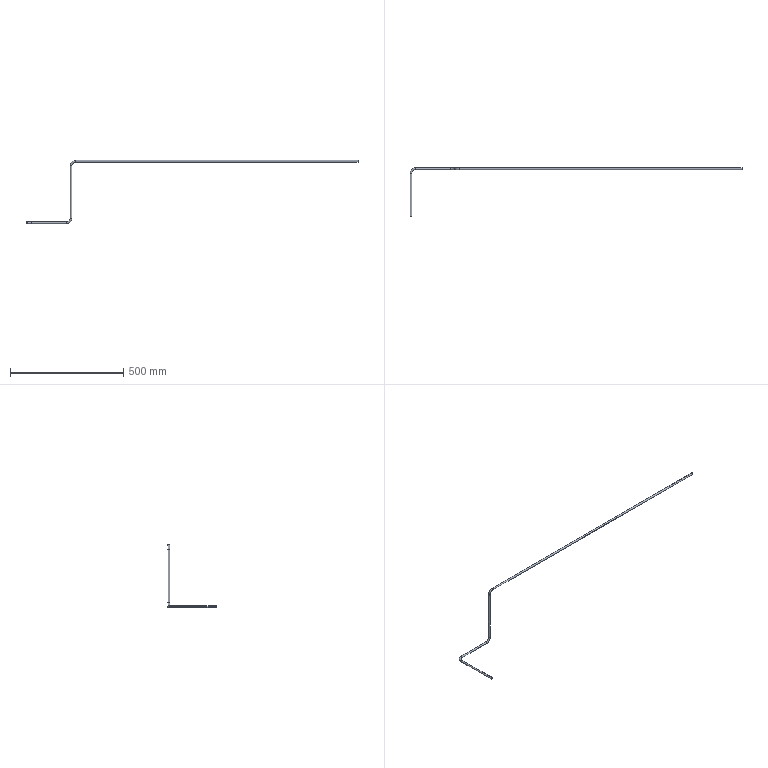Part | NX | features solid 2 | 1 solid | 16 faces | box 1467 x 214 x 279.213 mm | volume 82883 mm3 | cylinder 8 | torus 6 | plane 2 | commonest cylinder face diameters 3 x4 8 x4
STEP:
#1=CARTESIAN_POINT('',(-940.,-25.,-372.213));
#2=VERTEX_POINT('',#1);
#3=CARTESIAN_POINT('',(-940.,-25.,-376.213));
#4=DIRECTION('',(0.,-1.,0.));
#5=DIRECTION('',(0.,0.,1.));
#6=AXIS2_PLACEMENT_3D('',#3,#4,#5);
#7=CIRCLE('',#6,4.);
#8=EDGE_CURVE('',#2,#2,#7,.T.);
#9=ORIENTED_EDGE('',*,*,#8,.T.);
#10=EDGE_LOOP('',(#9));
#11=FACE_BOUND('',#10,.T.);
#12=CARTESIAN_POINT('',(-940.,-215.,-372.213));
#13=VERTEX_POINT('',#12);
#14=CARTESIAN_POINT('',(-940.,-215.,-376.213));
#15=DIRECTION('',(0.,-1.,0.));
#16=DIRECTION('',(0.,0.,1.));
#17=AXIS2_PLACEMENT_3D('',#14,#15,#16);
#18=CIRCLE('',#17,4.);
#19=EDGE_CURVE('',#13,#13,#18,.T.);
#20=ORIENTED_EDGE('',*,*,#19,.F.);
#21=EDGE_LOOP('',(#20));
#22=FACE_BOUND('',#21,.T.);
#23=CARTESIAN_POINT('',(-940.,-25.,-376.213));
#24=DIRECTION('',(0.,-1.,0.));
#25=DIRECTION('',(0.,0.,-1.));
#26=AXIS2_PLACEMENT_3D('',#23,#24,#25);
#27=CYLINDRICAL_SURFACE('',#26,4.);
#28=ADVANCED_FACE('',(#11,#22),#27,.T.);
#29=CARTESIAN_POINT('',(-940.,-25.,-374.713));
#30=VERTEX_POINT('',#29);
#31=CARTESIAN_POINT('',(-940.,-25.,-376.213));
#32=DIRECTION('',(0.,-1.,0.));
#33=DIRECTION('',(0.,0.,1.));
#34=AXIS2_PLACEMENT_3D('',#31,#32,#33);
#35=CIRCLE('',#34,1.5);
#36=EDGE_CURVE('',#30,#30,#35,.T.);
#37=ORIENTED_EDGE('',*,*,#36,.F.);
#38=EDGE_LOOP('',(#37));
#39=FACE_BOUND('',#38,.T.);
#40=CARTESIAN_POINT('',(-940.,-215.,-374.713));
#41=VERTEX_POINT('',#40);
#42=CARTESIAN_POINT('',(-940.,-215.,-376.213));
#43=DIRECTION('',(0.,-1.,0.));
#44=DIRECTION('',(0.,0.,1.));
#45=AXIS2_PLACEMENT_3D('',#42,#43,#44);
#46=CIRCLE('',#45,1.5);
#47=EDGE_CURVE('',#41,#41,#46,.T.);
#48=ORIENTED_EDGE('',*,*,#47,.T.);
#49=EDGE_LOOP('',(#48));
#50=FACE_BOUND('',#49,.T.);
#51=CARTESIAN_POINT('',(-940.,-25.,-376.213));
#52=DIRECTION('',(0.,-1.,0.));
#53=DIRECTION('',(0.,0.,-1.));
#54=AXIS2_PLACEMENT_3D('',#51,#52,#53);
#55=CYLINDRICAL_SURFACE('',#54,1.5);
#56=ADVANCED_FACE('',(#39,#50),#55,.F.);
#57=CARTESIAN_POINT('',(-920.,-5.,-372.213));
#58=VERTEX_POINT('',#57);
#59=CARTESIAN_POINT('',(-920.,-5.,-376.213));
#60=DIRECTION('',(-1.,0.,0.));
#61=DIRECTION('',(0.,0.,1.));
#62=AXIS2_PLACEMENT_3D('',#59,#60,#61);
#63=CIRCLE('',#62,4.);
#64=EDGE_CURVE('',#58,#58,#63,.T.);
#65=ORIENTED_EDGE('',*,*,#64,.T.);
#66=EDGE_LOOP('',(#65));
#67=FACE_BOUND('',#66,.T.);
#68=ORIENTED_EDGE('',*,*,#8,.F.);
#69=EDGE_LOOP('',(#68));
#70=FACE_BOUND('',#69,.T.);
#71=CARTESIAN_POINT('',(-920.,-25.,-376.213));
#72=DIRECTION('',(0.,0.,1.));
#73=DIRECTION('',(1.,0.,0.));
#74=AXIS2_PLACEMENT_3D('',#71,#72,#73);
#75=TOROIDAL_SURFACE('',#74,20.,4.);
#76=ADVANCED_FACE('',(#67,#70),#75,.T.);
#77=CARTESIAN_POINT('',(-920.,-5.,-374.713));
#78=VERTEX_POINT('',#77);
#79=CARTESIAN_POINT('',(-920.,-5.,-376.213));
#80=DIRECTION('',(-1.,0.,0.));
#81=DIRECTION('',(0.,0.,1.));
#82=AXIS2_PLACEMENT_3D('',#79,#80,#81);
#83=CIRCLE('',#82,1.5);
#84=EDGE_CURVE('',#78,#78,#83,.T.);
#85=ORIENTED_EDGE('',*,*,#84,.F.);
#86=EDGE_LOOP('',(#85));
#87=FACE_BOUND('',#86,.T.);
#88=ORIENTED_EDGE('',*,*,#36,.T.);
#89=EDGE_LOOP('',(#88));
#90=FACE_BOUND('',#89,.T.);
#91=CARTESIAN_POINT('',(-920.,-25.,-376.213));
#92=DIRECTION('',(0.,0.,1.));
#93=DIRECTION('',(1.,0.,0.));
#94=AXIS2_PLACEMENT_3D('',#91,#92,#93);
#95=TOROIDAL_SURFACE('',#94,20.,1.5);
#96=ADVANCED_FACE('',(#87,#90),#95,.F.);
#97=CARTESIAN_POINT('',(-765.,-5.,-372.213));
#98=VERTEX_POINT('',#97);
#99=CARTESIAN_POINT('',(-765.,-5.,-376.213));
#100=DIRECTION('',(-1.,0.,0.));
#101=DIRECTION('',(0.,0.,1.));
#102=AXIS2_PLACEMENT_3D('',#99,#100,#101);
#103=CIRCLE('',#102,4.);
#104=EDGE_CURVE('',#98,#98,#103,.T.);
#105=ORIENTED_EDGE('',*,*,#104,.T.);
#106=EDGE_LOOP('',(#105));
#107=FACE_BOUND('',#106,.T.);
#108=ORIENTED_EDGE('',*,*,#64,.F.);
#109=EDGE_LOOP('',(#108));
#110=FACE_BOUND('',#109,.T.);
#111=CARTESIAN_POINT('',(-765.,-5.,-376.213));
#112=DIRECTION('',(-1.,0.,0.));
#113=DIRECTION('',(0.,0.,1.));
#114=AXIS2_PLACEMENT_3D('',#111,#112,#113);
#115=CYLINDRICAL_SURFACE('',#114,4.);
#116=ADVANCED_FACE('',(#107,#110),#115,.T.);
#117=CARTESIAN_POINT('',(-765.,-5.,-374.713));
#118=VERTEX_POINT('',#117);
#119=CARTESIAN_POINT('',(-765.,-5.,-376.213));
#120=DIRECTION('',(-1.,0.,0.));
#121=DIRECTION('',(0.,0.,1.));
#122=AXIS2_PLACEMENT_3D('',#119,#120,#121);
#123=CIRCLE('',#122,1.5);
#124=EDGE_CURVE('',#118,#118,#123,.T.);
#125=ORIENTED_EDGE('',*,*,#124,.F.);
#126=EDGE_LOOP('',(#125));
#127=FACE_BOUND('',#126,.T.);
#128=ORIENTED_EDGE('',*,*,#84,.T.);
#129=EDGE_LOOP('',(#128));
#130=FACE_BOUND('',#129,.T.);
#131=CARTESIAN_POINT('',(-765.,-5.,-376.213));
#132=DIRECTION('',(-1.,0.,0.));
#133=DIRECTION('',(0.,0.,1.));
#134=AXIS2_PLACEMENT_3D('',#131,#132,#133);
#135=CYLINDRICAL_SURFACE('',#134,1.5);
#136=ADVANCED_FACE('',(#127,#130),#135,.F.);
#137=CARTESIAN_POINT('',(-749.,-5.,-356.213));
#138=VERTEX_POINT('',#137);
#139=CARTESIAN_POINT('',(-745.,-5.,-356.213));
#140=DIRECTION('',(0.,0.,-1.));
#141=DIRECTION('',(-1.,0.,0.));
#142=AXIS2_PLACEMENT_3D('',#139,#140,#141);
#143=CIRCLE('',#142,4.);
#144=EDGE_CURVE('',#138,#138,#143,.T.);
#145=ORIENTED_EDGE('',*,*,#144,.T.);
#146=EDGE_LOOP('',(#145));
#147=FACE_BOUND('',#146,.T.);
#148=ORIENTED_EDGE('',*,*,#104,.F.);
#149=EDGE_LOOP('',(#148));
#150=FACE_BOUND('',#149,.T.);
#151=CARTESIAN_POINT('',(-765.,-5.,-356.213));
#152=DIRECTION('',(0.,1.,0.));
#153=DIRECTION('',(0.,0.,1.));
#154=AXIS2_PLACEMENT_3D('',#151,#152,#153);
#155=TOROIDAL_SURFACE('',#154,20.,4.);
#156=ADVANCED_FACE('',(#147,#150),#155,.T.);
#157=CARTESIAN_POINT('',(-746.5,-5.,-356.213));
#158=VERTEX_POINT('',#157);
#159=CARTESIAN_POINT('',(-745.,-5.,-356.213));
#160=DIRECTION('',(0.,0.,-1.));
#161=DIRECTION('',(-1.,0.,0.));
#162=AXIS2_PLACEMENT_3D('',#159,#160,#161);
#163=CIRCLE('',#162,1.5);
#164=EDGE_CURVE('',#158,#158,#163,.T.);
#165=ORIENTED_EDGE('',*,*,#164,.F.);
#166=EDGE_LOOP('',(#165));
#167=FACE_BOUND('',#166,.T.);
#168=ORIENTED_EDGE('',*,*,#124,.T.);
#169=EDGE_LOOP('',(#168));
#170=FACE_BOUND('',#169,.T.);
#171=CARTESIAN_POINT('',(-765.,-5.,-356.213));
#172=DIRECTION('',(0.,1.,0.));
#173=DIRECTION('',(0.,0.,1.));
#174=AXIS2_PLACEMENT_3D('',#171,#172,#173);
#175=TOROIDAL_SURFACE('',#174,20.,1.5);
#176=ADVANCED_FACE('',(#167,#170),#175,.F.);
#177=CARTESIAN_POINT('',(-749.,-5.,-125.));
#178=VERTEX_POINT('',#177);
#179=CARTESIAN_POINT('',(-745.,-5.,-125.));
#180=DIRECTION('',(0.,0.,-1.));
#181=DIRECTION('',(-1.,0.,0.));
#182=AXIS2_PLACEMENT_3D('',#179,#180,#181);
#183=CIRCLE('',#182,4.);
#184=EDGE_CURVE('',#178,#178,#183,.T.);
#185=ORIENTED_EDGE('',*,*,#184,.T.);
#186=EDGE_LOOP('',(#185));
#187=FACE_BOUND('',#186,.T.);
#188=ORIENTED_EDGE('',*,*,#144,.F.);
#189=EDGE_LOOP('',(#188));
#190=FACE_BOUND('',#189,.T.);
#191=CARTESIAN_POINT('',(-745.,-5.,-125.));
#192=DIRECTION('',(0.,0.,-1.));
#193=DIRECTION('',(-1.,0.,0.));
#194=AXIS2_PLACEMENT_3D('',#191,#192,#193);
#195=CYLINDRICAL_SURFACE('',#194,4.);
#196=ADVANCED_FACE('',(#187,#190),#195,.T.);
#197=CARTESIAN_POINT('',(-746.5,-5.,-125.));
#198=VERTEX_POINT('',#197);
#199=CARTESIAN_POINT('',(-745.,-5.,-125.));
#200=DIRECTION('',(0.,0.,-1.));
#201=DIRECTION('',(-1.,0.,0.));
#202=AXIS2_PLACEMENT_3D('',#199,#200,#201);
#203=CIRCLE('',#202,1.5);
#204=EDGE_CURVE('',#198,#198,#203,.T.);
#205=ORIENTED_EDGE('',*,*,#204,.F.);
#206=EDGE_LOOP('',(#205));
#207=FACE_BOUND('',#206,.T.);
#208=ORIENTED_EDGE('',*,*,#164,.T.);
#209=EDGE_LOOP('',(#208));
#210=FACE_BOUND('',#209,.T.);
#211=CARTESIAN_POINT('',(-745.,-5.,-125.));
#212=DIRECTION('',(0.,0.,-1.));
#213=DIRECTION('',(-1.,0.,0.));
#214=AXIS2_PLACEMENT_3D('',#211,#212,#213);
#215=CYLINDRICAL_SURFACE('',#214,1.5);
#216=ADVANCED_FACE('',(#207,#210),#215,.F.);
#217=CARTESIAN_POINT('',(-725.,-5.,-101.));
#218=VERTEX_POINT('',#217);
#219=CARTESIAN_POINT('',(-725.,-5.,-105.));
#220=DIRECTION('',(-1.,0.,0.));
#221=DIRECTION('',(0.,0.,1.));
#222=AXIS2_PLACEMENT_3D('',#219,#220,#221);
#223=CIRCLE('',#222,4.);
#224=EDGE_CURVE('',#218,#218,#223,.T.);
#225=ORIENTED_EDGE('',*,*,#224,.T.);
#226=EDGE_LOOP('',(#225));
#227=FACE_BOUND('',#226,.T.);
#228=ORIENTED_EDGE('',*,*,#184,.F.);
#229=EDGE_LOOP('',(#228));
#230=FACE_BOUND('',#229,.T.);
#231=CARTESIAN_POINT('',(-725.,-5.,-125.));
#232=DIRECTION('',(0.,-1.,0.));
#233=DIRECTION('',(0.,0.,-1.));
#234=AXIS2_PLACEMENT_3D('',#231,#232,#233);
#235=TOROIDAL_SURFACE('',#234,20.,4.);
#236=ADVANCED_FACE('',(#227,#230),#235,.T.);
#237=CARTESIAN_POINT('',(-725.,-5.,-103.5));
#238=VERTEX_POINT('',#237);
#239=CARTESIAN_POINT('',(-725.,-5.,-105.));
#240=DIRECTION('',(-1.,0.,0.));
#241=DIRECTION('',(0.,0.,1.));
#242=AXIS2_PLACEMENT_3D('',#239,#240,#241);
#243=CIRCLE('',#242,1.5);
#244=EDGE_CURVE('',#238,#238,#243,.T.);
#245=ORIENTED_EDGE('',*,*,#244,.F.);
#246=EDGE_LOOP('',(#245));
#247=FACE_BOUND('',#246,.T.);
#248=ORIENTED_EDGE('',*,*,#204,.T.);
#249=EDGE_LOOP('',(#248));
#250=FACE_BOUND('',#249,.T.);
#251=CARTESIAN_POINT('',(-725.,-5.,-125.));
#252=DIRECTION('',(0.,-1.,0.));
#253=DIRECTION('',(0.,0.,-1.));
#254=AXIS2_PLACEMENT_3D('',#251,#252,#253);
#255=TOROIDAL_SURFACE('',#254,20.,1.5);
#256=ADVANCED_FACE('',(#247,#250),#255,.F.);
#257=ORIENTED_EDGE('',*,*,#244,.T.);
#258=EDGE_LOOP('',(#257));
#259=FACE_BOUND('',#258,.T.);
#260=CARTESIAN_POINT('',(523.271,-5.,-103.5));
#261=VERTEX_POINT('',#260);
#262=CARTESIAN_POINT('',(523.271,-5.,-105.));
#263=DIRECTION('',(-1.,0.,0.));
#264=DIRECTION('',(0.,0.,1.));
#265=AXIS2_PLACEMENT_3D('',#262,#263,#264);
#266=CIRCLE('',#265,1.5);
#267=EDGE_CURVE('',#261,#261,#266,.T.);
#268=ORIENTED_EDGE('',*,*,#267,.F.);
#269=EDGE_LOOP('',(#268));
#270=FACE_BOUND('',#269,.T.);
#271=CARTESIAN_POINT('',(-725.,-5.,-105.));
#272=DIRECTION('',(1.,0.,0.));
#273=DIRECTION('',(0.,0.,-1.));
#274=AXIS2_PLACEMENT_3D('',#271,#272,#273);
#275=CYLINDRICAL_SURFACE('',#274,1.5);
#276=ADVANCED_FACE('',(#259,#270),#275,.F.);
#277=ORIENTED_EDGE('',*,*,#224,.F.);
#278=EDGE_LOOP('',(#277));
#279=FACE_BOUND('',#278,.T.);
#280=CARTESIAN_POINT('',(523.271,-5.,-101.));
#281=VERTEX_POINT('',#280);
#282=CARTESIAN_POINT('',(523.271,-5.,-105.));
#283=DIRECTION('',(-1.,0.,0.));
#284=DIRECTION('',(0.,0.,1.));
#285=AXIS2_PLACEMENT_3D('',#282,#283,#284);
#286=CIRCLE('',#285,4.);
#287=EDGE_CURVE('',#281,#281,#286,.T.);
#288=ORIENTED_EDGE('',*,*,#287,.T.);
#289=EDGE_LOOP('',(#288));
#290=FACE_BOUND('',#289,.T.);
#291=CARTESIAN_POINT('',(-725.,-5.,-105.));
#292=DIRECTION('',(1.,0.,0.));
#293=DIRECTION('',(0.,0.,-1.));
#294=AXIS2_PLACEMENT_3D('',#291,#292,#293);
#295=CYLINDRICAL_SURFACE('',#294,4.);
#296=ADVANCED_FACE('',(#279,#290),#295,.T.);
#297=ORIENTED_EDGE('',*,*,#47,.F.);
#298=EDGE_LOOP('',(#297));
#299=FACE_BOUND('',#298,.T.);
#300=ORIENTED_EDGE('',*,*,#19,.T.);
#301=EDGE_LOOP('',(#300));
#302=FACE_BOUND('',#301,.T.);
#303=CARTESIAN_POINT('',(-940.,-215.,-376.213));
#304=DIRECTION('',(0.,-1.,0.));
#305=DIRECTION('',(0.,0.,1.));
#306=AXIS2_PLACEMENT_3D('',#303,#304,#305);
#307=PLANE('',#306);
#308=ADVANCED_FACE('',(#299,#302),#307,.T.);
#309=ORIENTED_EDGE('',*,*,#267,.T.);
#310=EDGE_LOOP('',(#309));
#311=FACE_BOUND('',#310,.T.);
#312=ORIENTED_EDGE('',*,*,#287,.F.);
#313=EDGE_LOOP('',(#312));
#314=FACE_BOUND('',#313,.T.);
#315=CARTESIAN_POINT('',(523.271,-5.,-105.));
#316=DIRECTION('',(-1.,0.,0.));
#317=DIRECTION('',(0.,0.,1.));
#318=AXIS2_PLACEMENT_3D('',#315,#316,#317);
#319=PLANE('',#318);
#320=ADVANCED_FACE('',(#311,#314),#319,.F.);
#321=CLOSED_SHELL('',(#28,#56,#76,#96,#116,#136,#156,#176,#196,#216,#236,#256,#276,#296,#308,#320));
#322=MANIFOLD_SOLID_BREP('',#321);
#323=(LENGTH_UNIT()NAMED_UNIT(*)SI_UNIT(.MILLI.,.METRE.));
#324=UNCERTAINTY_MEASURE_WITH_UNIT(LENGTH_MEASURE(0.00001),#323,'','');
#325=(NAMED_UNIT(*)PLANE_ANGLE_UNIT()SI_UNIT($,.RADIAN.));
#326=(NAMED_UNIT(*)SI_UNIT($,.STERADIAN.)SOLID_ANGLE_UNIT());
#327=(GEOMETRIC_REPRESENTATION_CONTEXT(3)GLOBAL_UNCERTAINTY_ASSIGNED_CONTEXT((#324))GLOBAL_UNIT_ASSIGNED_CONTEXT((#323,#325,#326))REPRESENTATION_CONTEXT('',''));
#328=ADVANCED_BREP_SHAPE_REPRESENTATION('',(#322),#327);